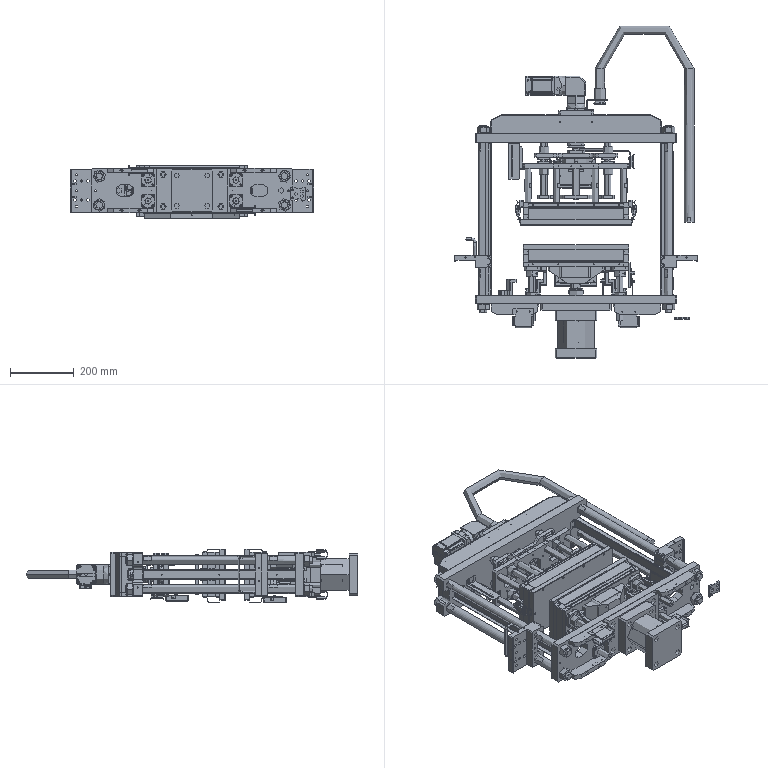Part | SolidWorks | 172 solids | 10397 faces | volume 2156795733372051217872648900772085811361186091496738347275634360435010736762998889556743347217459279804146683613061124027188862765683868812777387331615309057739783667712 mm3 | cylinder 4705 | plane 4153 | cone 1223 | torus 164 | spline 118 | sphere 34 | commonest cylinder face diameters 4 x328 5 x282 6 x258 6.6 x224 3.3 x204 11 x192